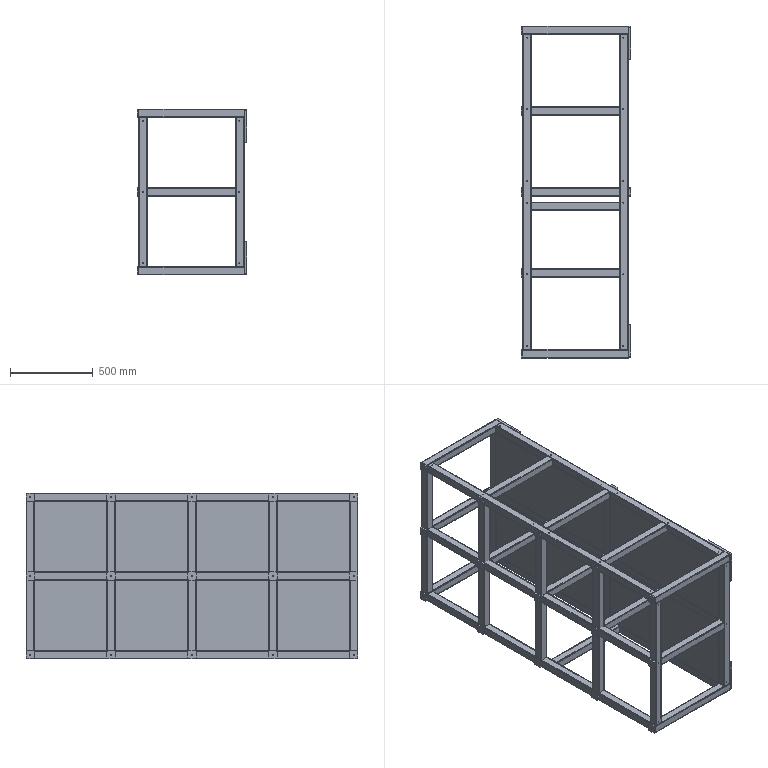Part | SolidWorks | features Fillet 21, HoleWzd 17, WeldCornerFeat 11, ICE 6, Chamfer 4, WeldMemberFeat 3, 3DProfileFeature 1, MoveFace 1, WeldmentFeature 1 | 56 solids | 966 faces | box 660 x 2000 x 1000 mm | volume 17994885 mm3 | cylinder 496 | plane 470 | commonest cylinder face diameters 8 x132 3 x124 5 x80 8.5 x58 10 x48 6.8 x32